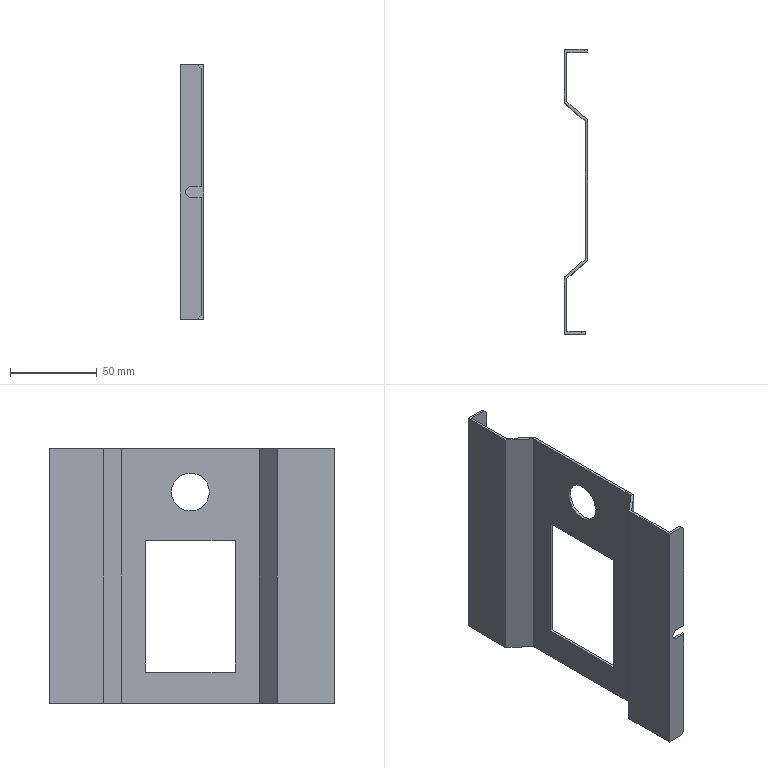Part | SolidWorks | features ICE 4, Chamfer 1, ExtruThin 1, MirrorPattern 1 | 1 solid | 36 faces | box 13.5 x 164.498 x 147 mm | volume 37040 mm3 | plane 29 | cylinder 7 | commonest cylinder face diameters 4.5 x4 22 x2 6 x1
STEP:
#1=CARTESIAN_POINT('',(9.75,162.998,35.));
#2=VERTEX_POINT('',#1);
#3=CARTESIAN_POINT('',(5.25,162.998,35.));
#4=VERTEX_POINT('',#3);
#5=CARTESIAN_POINT('',(7.5,162.998,35.));
#6=DIRECTION('',(0.,1.,0.));
#7=DIRECTION('',(1.,0.,0.));
#8=AXIS2_PLACEMENT_3D('',#5,#6,#7);
#9=CIRCLE('',#8,2.25);
#10=EDGE_CURVE('',#2,#4,#9,.T.);
#11=ORIENTED_EDGE('',*,*,#10,.F.);
#12=CARTESIAN_POINT('',(9.75,164.498,35.));
#13=VERTEX_POINT('',#12);
#14=CARTESIAN_POINT('',(9.75,154.498,35.));
#15=DIRECTION('',(0.,1.,0.));
#16=VECTOR('',#15,1000.);
#17=LINE('',#14,#16);
#18=EDGE_CURVE('',#2,#13,#17,.T.);
#19=ORIENTED_EDGE('',*,*,#18,.T.);
#20=CARTESIAN_POINT('',(5.25,164.498,35.));
#21=VERTEX_POINT('',#20);
#22=CARTESIAN_POINT('',(7.5,164.498,35.));
#23=DIRECTION('',(0.,-1.,0.));
#24=DIRECTION('',(-1.,0.,0.));
#25=AXIS2_PLACEMENT_3D('',#22,#23,#24);
#26=CIRCLE('',#25,2.25);
#27=EDGE_CURVE('',#21,#13,#26,.T.);
#28=ORIENTED_EDGE('',*,*,#27,.F.);
#29=CARTESIAN_POINT('',(5.25,154.498,35.));
#30=DIRECTION('',(0.,1.,0.));
#31=VECTOR('',#30,1000.);
#32=LINE('',#29,#31);
#33=EDGE_CURVE('',#4,#21,#32,.T.);
#34=ORIENTED_EDGE('',*,*,#33,.F.);
#35=EDGE_LOOP('',(#11,#19,#28,#34));
#36=FACE_OUTER_BOUND('',#35,.T.);
#37=CARTESIAN_POINT('',(7.5,154.498,35.));
#38=DIRECTION('',(0.,1.,0.));
#39=DIRECTION('',(-1.,0.,0.));
#40=AXIS2_PLACEMENT_3D('',#37,#38,#39);
#41=CYLINDRICAL_SURFACE('',#40,2.25);
#42=ADVANCED_FACE('',(#36),#41,.F.);
#43=CARTESIAN_POINT('',(5.25,162.998,-35.));
#44=VERTEX_POINT('',#43);
#45=CARTESIAN_POINT('',(9.75,162.998,-35.));
#46=VERTEX_POINT('',#45);
#47=CARTESIAN_POINT('',(7.5,162.998,-35.));
#48=DIRECTION('',(0.,-1.,0.));
#49=DIRECTION('',(1.,0.,0.));
#50=AXIS2_PLACEMENT_3D('',#47,#48,#49);
#51=CIRCLE('',#50,2.25);
#52=EDGE_CURVE('',#44,#46,#51,.T.);
#53=ORIENTED_EDGE('',*,*,#52,.T.);
#54=CARTESIAN_POINT('',(9.75,164.498,-35.));
#55=VERTEX_POINT('',#54);
#56=CARTESIAN_POINT('',(9.75,154.498,-35.));
#57=DIRECTION('',(0.,1.,0.));
#58=VECTOR('',#57,1000.);
#59=LINE('',#56,#58);
#60=EDGE_CURVE('',#46,#55,#59,.T.);
#61=ORIENTED_EDGE('',*,*,#60,.T.);
#62=CARTESIAN_POINT('',(5.25,164.498,-35.));
#63=VERTEX_POINT('',#62);
#64=CARTESIAN_POINT('',(7.5,164.498,-35.));
#65=DIRECTION('',(0.,1.,0.));
#66=DIRECTION('',(-1.,0.,0.));
#67=AXIS2_PLACEMENT_3D('',#64,#65,#66);
#68=CIRCLE('',#67,2.25);
#69=EDGE_CURVE('',#55,#63,#68,.T.);
#70=ORIENTED_EDGE('',*,*,#69,.T.);
#71=CARTESIAN_POINT('',(5.25,154.498,-35.));
#72=DIRECTION('',(0.,1.,0.));
#73=VECTOR('',#72,1000.);
#74=LINE('',#71,#73);
#75=EDGE_CURVE('',#44,#63,#74,.T.);
#76=ORIENTED_EDGE('',*,*,#75,.F.);
#77=EDGE_LOOP('',(#53,#61,#70,#76));
#78=FACE_OUTER_BOUND('',#77,.T.);
#79=CARTESIAN_POINT('',(7.5,154.498,-35.));
#80=DIRECTION('',(0.,1.,0.));
#81=DIRECTION('',(-1.,0.,0.));
#82=AXIS2_PLACEMENT_3D('',#79,#80,#81);
#83=CYLINDRICAL_SURFACE('',#82,2.25);
#84=ADVANCED_FACE('',(#78),#83,.F.);
#85=CARTESIAN_POINT('',(13.5,72.249,48.5));
#86=VERTEX_POINT('',#85);
#87=CARTESIAN_POINT('',(13.5,94.249,48.5));
#88=VERTEX_POINT('',#87);
#89=CARTESIAN_POINT('',(13.5,83.249,48.5));
#90=DIRECTION('',(1.,0.,0.));
#91=DIRECTION('',(0.,1.,0.));
#92=AXIS2_PLACEMENT_3D('',#89,#90,#91);
#93=CIRCLE('',#92,11.);
#94=EDGE_CURVE('',#86,#88,#93,.T.);
#95=ORIENTED_EDGE('',*,*,#94,.T.);
#96=CARTESIAN_POINT('',(12.,94.249,48.5));
#97=VERTEX_POINT('',#96);
#98=CARTESIAN_POINT('',(22.,94.249,48.5));
#99=DIRECTION('',(-1.,0.,0.));
#100=VECTOR('',#99,1000.);
#101=LINE('',#98,#100);
#102=EDGE_CURVE('',#88,#97,#101,.T.);
#103=ORIENTED_EDGE('',*,*,#102,.T.);
#104=CARTESIAN_POINT('',(12.,72.249,48.5));
#105=VERTEX_POINT('',#104);
#106=CARTESIAN_POINT('',(12.,83.249,48.5));
#107=DIRECTION('',(-1.,0.,0.));
#108=DIRECTION('',(0.,-1.,0.));
#109=AXIS2_PLACEMENT_3D('',#106,#107,#108);
#110=CIRCLE('',#109,11.);
#111=EDGE_CURVE('',#97,#105,#110,.T.);
#112=ORIENTED_EDGE('',*,*,#111,.T.);
#113=CARTESIAN_POINT('',(22.,72.249,48.5));
#114=DIRECTION('',(-1.,0.,0.));
#115=VECTOR('',#114,1000.);
#116=LINE('',#113,#115);
#117=EDGE_CURVE('',#86,#105,#116,.T.);
#118=ORIENTED_EDGE('',*,*,#117,.F.);
#119=EDGE_LOOP('',(#95,#103,#112,#118));
#120=FACE_OUTER_BOUND('',#119,.T.);
#121=CARTESIAN_POINT('',(22.,83.249,48.5));
#122=DIRECTION('',(-1.,0.,0.));
#123=DIRECTION('',(0.,-1.,0.));
#124=AXIS2_PLACEMENT_3D('',#121,#122,#123);
#125=CYLINDRICAL_SURFACE('',#124,11.);
#126=ADVANCED_FACE('',(#120),#125,.F.);
#127=CARTESIAN_POINT('',(11.5,162.998,-73.5));
#128=VERTEX_POINT('',#127);
#129=CARTESIAN_POINT('',(1.5,162.998,-73.5));
#130=VERTEX_POINT('',#129);
#131=CARTESIAN_POINT('',(0.,162.998,-73.5));
#132=DIRECTION('',(-1.,0.,0.));
#133=VECTOR('',#132,1000.);
#134=LINE('',#131,#133);
#135=EDGE_CURVE('',#128,#130,#134,.T.);
#136=ORIENTED_EDGE('',*,*,#135,.F.);
#137=CARTESIAN_POINT('',(13.5,162.998,-71.5));
#138=VERTEX_POINT('',#137);
#139=CARTESIAN_POINT('',(79.25,162.998,-5.75));
#140=DIRECTION('',(0.7071,0.,0.7071));
#141=VECTOR('',#140,1000.);
#142=LINE('',#139,#141);
#143=EDGE_CURVE('',#128,#138,#142,.T.);
#144=ORIENTED_EDGE('',*,*,#143,.T.);
#145=CARTESIAN_POINT('',(13.5,162.998,71.5));
#146=VERTEX_POINT('',#145);
#147=CARTESIAN_POINT('',(13.5,162.998,73.5));
#148=DIRECTION('',(0.,0.,-1.));
#149=VECTOR('',#148,1000.);
#150=LINE('',#147,#149);
#151=EDGE_CURVE('',#146,#138,#150,.T.);
#152=ORIENTED_EDGE('',*,*,#151,.F.);
#153=CARTESIAN_POINT('',(11.5,162.998,73.5));
#154=VERTEX_POINT('',#153);
#155=CARTESIAN_POINT('',(5.75,162.998,79.25));
#156=DIRECTION('',(-0.7071,0.,0.7071));
#157=VECTOR('',#156,1000.);
#158=LINE('',#155,#157);
#159=EDGE_CURVE('',#146,#154,#158,.T.);
#160=ORIENTED_EDGE('',*,*,#159,.T.);
#161=CARTESIAN_POINT('',(1.5,162.998,73.5));
#162=VERTEX_POINT('',#161);
#163=CARTESIAN_POINT('',(0.,162.998,73.5));
#164=DIRECTION('',(-1.,0.,0.));
#165=VECTOR('',#164,1000.);
#166=LINE('',#163,#165);
#167=EDGE_CURVE('',#154,#162,#166,.T.);
#168=ORIENTED_EDGE('',*,*,#167,.T.);
#169=CARTESIAN_POINT('',(1.5,162.998,73.5));
#170=DIRECTION('',(0.,0.,-1.));
#171=VECTOR('',#170,1000.);
#172=LINE('',#169,#171);
#173=EDGE_CURVE('',#162,#130,#172,.T.);
#174=ORIENTED_EDGE('',*,*,#173,.T.);
#175=EDGE_LOOP('',(#136,#144,#152,#160,#168,#174));
#176=FACE_OUTER_BOUND('',#175,.T.);
#177=ORIENTED_EDGE('',*,*,#52,.F.);
#178=CARTESIAN_POINT('',(7.5,162.998,-35.));
#179=DIRECTION('',(0.,-1.,0.));
#180=DIRECTION('',(1.,0.,0.));
#181=AXIS2_PLACEMENT_3D('',#178,#179,#180);
#182=CIRCLE('',#181,2.25);
#183=EDGE_CURVE('',#46,#44,#182,.T.);
#184=ORIENTED_EDGE('',*,*,#183,.F.);
#185=EDGE_LOOP('',(#177,#184));
#186=FACE_BOUND('',#185,.T.);
#187=CARTESIAN_POINT('',(7.5,162.998,35.));
#188=DIRECTION('',(0.,1.,0.));
#189=DIRECTION('',(1.,0.,0.));
#190=AXIS2_PLACEMENT_3D('',#187,#188,#189);
#191=CIRCLE('',#190,2.25);
#192=EDGE_CURVE('',#4,#2,#191,.T.);
#193=ORIENTED_EDGE('',*,*,#192,.T.);
#194=ORIENTED_EDGE('',*,*,#10,.T.);
#195=EDGE_LOOP('',(#193,#194));
#196=FACE_BOUND('',#195,.T.);
#197=CARTESIAN_POINT('',(0.,162.998,73.5));
#198=DIRECTION('',(0.,-1.,0.));
#199=DIRECTION('',(1.,0.,0.));
#200=AXIS2_PLACEMENT_3D('',#197,#198,#199);
#201=PLANE('',#200);
#202=ADVANCED_FACE('',(#176,#186,#196),#201,.T.);
#203=CARTESIAN_POINT('',(13.5,164.498,71.5));
#204=VERTEX_POINT('',#203);
#205=CARTESIAN_POINT('',(13.5,164.498,-71.5));
#206=VERTEX_POINT('',#205);
#207=CARTESIAN_POINT('',(13.5,164.498,73.5));
#208=DIRECTION('',(0.,0.,-1.));
#209=VECTOR('',#208,1000.);
#210=LINE('',#207,#209);
#211=EDGE_CURVE('',#204,#206,#210,.T.);
#212=ORIENTED_EDGE('',*,*,#211,.T.);
#213=CARTESIAN_POINT('',(11.5,164.498,-73.5));
#214=VERTEX_POINT('',#213);
#215=CARTESIAN_POINT('',(11.5,164.498,-73.5));
#216=DIRECTION('',(-0.7071,0.,-0.7071));
#217=VECTOR('',#216,1000.);
#218=LINE('',#215,#217);
#219=EDGE_CURVE('',#206,#214,#218,.T.);
#220=ORIENTED_EDGE('',*,*,#219,.T.);
#221=CARTESIAN_POINT('',(0.,164.498,-73.5));
#222=VERTEX_POINT('',#221);
#223=CARTESIAN_POINT('',(0.,164.498,-73.5));
#224=DIRECTION('',(-1.,0.,0.));
#225=VECTOR('',#224,1000.);
#226=LINE('',#223,#225);
#227=EDGE_CURVE('',#214,#222,#226,.T.);
#228=ORIENTED_EDGE('',*,*,#227,.T.);
#229=CARTESIAN_POINT('',(0.,164.498,73.5));
#230=VERTEX_POINT('',#229);
#231=CARTESIAN_POINT('',(0.,164.498,73.5));
#232=DIRECTION('',(0.,0.,-1.));
#233=VECTOR('',#232,1000.);
#234=LINE('',#231,#233);
#235=EDGE_CURVE('',#230,#222,#234,.T.);
#236=ORIENTED_EDGE('',*,*,#235,.F.);
#237=CARTESIAN_POINT('',(11.5,164.498,73.5));
#238=VERTEX_POINT('',#237);
#239=CARTESIAN_POINT('',(0.,164.498,73.5));
#240=DIRECTION('',(-1.,0.,0.));
#241=VECTOR('',#240,1000.);
#242=LINE('',#239,#241);
#243=EDGE_CURVE('',#238,#230,#242,.T.);
#244=ORIENTED_EDGE('',*,*,#243,.F.);
#245=CARTESIAN_POINT('',(13.5,164.498,71.5));
#246=DIRECTION('',(0.7071,0.,-0.7071));
#247=VECTOR('',#246,1000.);
#248=LINE('',#245,#247);
#249=EDGE_CURVE('',#238,#204,#248,.T.);
#250=ORIENTED_EDGE('',*,*,#249,.T.);
#251=EDGE_LOOP('',(#212,#220,#228,#236,#244,#250));
#252=FACE_OUTER_BOUND('',#251,.T.);
#253=CARTESIAN_POINT('',(7.5,164.498,-35.));
#254=DIRECTION('',(0.,1.,0.));
#255=DIRECTION('',(-1.,0.,0.));
#256=AXIS2_PLACEMENT_3D('',#253,#254,#255);
#257=CIRCLE('',#256,2.25);
#258=EDGE_CURVE('',#63,#55,#257,.T.);
#259=ORIENTED_EDGE('',*,*,#258,.F.);
#260=ORIENTED_EDGE('',*,*,#69,.F.);
#261=EDGE_LOOP('',(#259,#260));
#262=FACE_BOUND('',#261,.T.);
#263=ORIENTED_EDGE('',*,*,#27,.T.);
#264=CARTESIAN_POINT('',(7.5,164.498,35.));
#265=DIRECTION('',(0.,-1.,0.));
#266=DIRECTION('',(-1.,0.,0.));
#267=AXIS2_PLACEMENT_3D('',#264,#265,#266);
#268=CIRCLE('',#267,2.25);
#269=EDGE_CURVE('',#13,#21,#268,.T.);
#270=ORIENTED_EDGE('',*,*,#269,.T.);
#271=EDGE_LOOP('',(#263,#270));
#272=FACE_BOUND('',#271,.T.);
#273=CARTESIAN_POINT('',(0.,164.498,73.5));
#274=DIRECTION('',(0.,-1.,0.));
#275=DIRECTION('',(1.,0.,0.));
#276=AXIS2_PLACEMENT_3D('',#273,#274,#275);
#277=PLANE('',#276);
#278=ADVANCED_FACE('',(#252,#262,#272),#277,.F.);
#279=CARTESIAN_POINT('',(12.,1.5,3.));
#280=VERTEX_POINT('',#279);
#281=CARTESIAN_POINT('',(12.,0.,3.));
#282=VERTEX_POINT('',#281);
#283=CARTESIAN_POINT('',(12.,5.,3.));
#284=DIRECTION('',(0.,-1.,0.));
#285=VECTOR('',#284,1000.);
#286=LINE('',#283,#285);
#287=EDGE_CURVE('',#280,#282,#286,.T.);
#288=ORIENTED_EDGE('',*,*,#287,.F.);
#289=CARTESIAN_POINT('',(12.,1.5,71.5));
#290=VERTEX_POINT('',#289);
#291=CARTESIAN_POINT('',(12.,1.5,73.5));
#292=DIRECTION('',(0.,0.,-1.));
#293=VECTOR('',#292,1000.);
#294=LINE('',#291,#293);
#295=EDGE_CURVE('',#290,#280,#294,.T.);
#296=ORIENTED_EDGE('',*,*,#295,.F.);
#297=CARTESIAN_POINT('',(12.,0.,71.5));
#298=VERTEX_POINT('',#297);
#299=CARTESIAN_POINT('',(12.,0.,71.5));
#300=DIRECTION('',(0.,-1.,0.));
#301=VECTOR('',#300,1000.);
#302=LINE('',#299,#301);
#303=EDGE_CURVE('',#290,#298,#302,.T.);
#304=ORIENTED_EDGE('',*,*,#303,.T.);
#305=CARTESIAN_POINT('',(12.,0.,73.5));
#306=DIRECTION('',(0.,0.,-1.));
#307=VECTOR('',#306,1000.);
#308=LINE('',#305,#307);
#309=EDGE_CURVE('',#298,#282,#308,.T.);
#310=ORIENTED_EDGE('',*,*,#309,.T.);
#311=EDGE_LOOP('',(#288,#296,#304,#310));
#312=FACE_OUTER_BOUND('',#311,.T.);
#313=CARTESIAN_POINT('',(12.,1.5,73.5));
#314=DIRECTION('',(1.,0.,0.));
#315=DIRECTION('',(0.,0.,-1.));
#316=AXIS2_PLACEMENT_3D('',#313,#314,#315);
#317=PLANE('',#316);
#318=ADVANCED_FACE('',(#312),#317,.T.);
#319=CARTESIAN_POINT('',(6.,0.,3.));
#320=VERTEX_POINT('',#319);
#321=CARTESIAN_POINT('',(6.,0.,-3.));
#322=VERTEX_POINT('',#321);
#323=CARTESIAN_POINT('',(6.,0.,0.));
#324=DIRECTION('',(0.,-1.,0.));
#325=DIRECTION('',(0.,0.,-1.));
#326=AXIS2_PLACEMENT_3D('',#323,#324,#325);
#327=CIRCLE('',#326,3.);
#328=EDGE_CURVE('',#320,#322,#327,.T.);
#329=ORIENTED_EDGE('',*,*,#328,.F.);
#330=CARTESIAN_POINT('',(6.,0.,3.));
#331=DIRECTION('',(-1.,0.,0.));
#332=VECTOR('',#331,1000.);
#333=LINE('',#330,#332);
#334=EDGE_CURVE('',#282,#320,#333,.T.);
#335=ORIENTED_EDGE('',*,*,#334,.F.);
#336=ORIENTED_EDGE('',*,*,#309,.F.);
#337=CARTESIAN_POINT('',(10.,0.,73.5));
#338=VERTEX_POINT('',#337);
#339=CARTESIAN_POINT('',(12.,0.,71.5));
#340=DIRECTION('',(-0.7071,0.,0.7071));
#341=VECTOR('',#340,1000.);
#342=LINE('',#339,#341);
#343=EDGE_CURVE('',#298,#338,#342,.T.);
#344=ORIENTED_EDGE('',*,*,#343,.T.);
#345=CARTESIAN_POINT('',(0.,0.,73.5));
#346=VERTEX_POINT('',#345);
#347=CARTESIAN_POINT('',(0.,0.,73.5));
#348=DIRECTION('',(1.,0.,0.));
#349=VECTOR('',#348,1000.);
#350=LINE('',#347,#349);
#351=EDGE_CURVE('',#346,#338,#350,.T.);
#352=ORIENTED_EDGE('',*,*,#351,.F.);
#353=CARTESIAN_POINT('',(0.,0.,-73.5));
#354=VERTEX_POINT('',#353);
#355=CARTESIAN_POINT('',(0.,0.,73.5));
#356=DIRECTION('',(0.,0.,-1.));
#357=VECTOR('',#356,1000.);
#358=LINE('',#355,#357);
#359=EDGE_CURVE('',#346,#354,#358,.T.);
#360=ORIENTED_EDGE('',*,*,#359,.T.);
#361=CARTESIAN_POINT('',(10.,0.,-73.5));
#362=VERTEX_POINT('',#361);
#363=CARTESIAN_POINT('',(0.,0.,-73.5));
#364=DIRECTION('',(1.,0.,0.));
#365=VECTOR('',#364,1000.);
#366=LINE('',#363,#365);
#367=EDGE_CURVE('',#354,#362,#366,.T.);
#368=ORIENTED_EDGE('',*,*,#367,.T.);
#369=CARTESIAN_POINT('',(12.,0.,-71.5));
#370=VERTEX_POINT('',#369);
#371=CARTESIAN_POINT('',(10.,0.,-73.5));
#372=DIRECTION('',(0.7071,0.,0.7071));
#373=VECTOR('',#372,1000.);
#374=LINE('',#371,#373);
#375=EDGE_CURVE('',#362,#370,#374,.T.);
#376=ORIENTED_EDGE('',*,*,#375,.T.);
#377=CARTESIAN_POINT('',(12.,0.,-3.));
#378=VERTEX_POINT('',#377);
#379=CARTESIAN_POINT('',(12.,0.,73.5));
#380=DIRECTION('',(0.,0.,-1.));
#381=VECTOR('',#380,1000.);
#382=LINE('',#379,#381);
#383=EDGE_CURVE('',#378,#370,#382,.T.);
#384=ORIENTED_EDGE('',*,*,#383,.F.);
#385=CARTESIAN_POINT('',(6.,0.,-3.));
#386=DIRECTION('',(1.,0.,0.));
#387=VECTOR('',#386,1000.);
#388=LINE('',#385,#387);
#389=EDGE_CURVE('',#322,#378,#388,.T.);
#390=ORIENTED_EDGE('',*,*,#389,.F.);
#391=EDGE_LOOP('',(#329,#335,#336,#344,#352,#360,#368,#376,#384,#390));
#392=FACE_OUTER_BOUND('',#391,.T.);
#393=CARTESIAN_POINT('',(0.,0.,73.5));
#394=DIRECTION('',(0.,1.,0.));
#395=DIRECTION('',(0.,0.,1.));
#396=AXIS2_PLACEMENT_3D('',#393,#394,#395);
#397=PLANE('',#396);
#398=ADVANCED_FACE('',(#392),#397,.F.);
#399=CARTESIAN_POINT('',(12.,1.5,-3.));
#400=VERTEX_POINT('',#399);
#401=CARTESIAN_POINT('',(12.,5.,-3.));
#402=DIRECTION('',(0.,-1.,0.));
#403=VECTOR('',#402,1000.);
#404=LINE('',#401,#403);
#405=EDGE_CURVE('',#400,#378,#404,.T.);
#406=ORIENTED_EDGE('',*,*,#405,.T.);
#407=ORIENTED_EDGE('',*,*,#383,.T.);
#408=CARTESIAN_POINT('',(12.,1.5,-71.5));
#409=VERTEX_POINT('',#408);
#410=CARTESIAN_POINT('',(12.,1.5,-71.5));
#411=DIRECTION('',(0.,1.,0.));
#412=VECTOR('',#411,1000.);
#413=LINE('',#410,#412);
#414=EDGE_CURVE('',#370,#409,#413,.T.);
#415=ORIENTED_EDGE('',*,*,#414,.T.);
#416=CARTESIAN_POINT('',(12.,1.5,73.5));
#417=DIRECTION('',(0.,0.,-1.));
#418=VECTOR('',#417,1000.);
#419=LINE('',#416,#418);
#420=EDGE_CURVE('',#400,#409,#419,.T.);
#421=ORIENTED_EDGE('',*,*,#420,.F.);
#422=EDGE_LOOP('',(#406,#407,#415,#421));
#423=FACE_OUTER_BOUND('',#422,.T.);
#424=CARTESIAN_POINT('',(12.,1.5,73.5));
#425=DIRECTION('',(1.,0.,0.));
#426=DIRECTION('',(0.,0.,-1.));
#427=AXIS2_PLACEMENT_3D('',#424,#425,#426);
#428=PLANE('',#427);
#429=ADVANCED_FACE('',(#423),#428,.T.);
#430=CARTESIAN_POINT('',(6.,1.5,3.));
#431=VERTEX_POINT('',#430);
#432=CARTESIAN_POINT('',(0.,1.5,3.));
#433=DIRECTION('',(1.,0.,0.));
#434=VECTOR('',#433,1000.);
#435=LINE('',#432,#434);
#436=EDGE_CURVE('',#431,#280,#435,.T.);
#437=ORIENTED_EDGE('',*,*,#436,.F.);
#438=CARTESIAN_POINT('',(6.,1.5,-3.));
#439=VERTEX_POINT('',#438);
#440=CARTESIAN_POINT('',(6.,1.5,0.));
#441=DIRECTION('',(0.,1.,0.));
#442=DIRECTION('',(0.,0.,1.));
#443=AXIS2_PLACEMENT_3D('',#440,#441,#442);
#444=CIRCLE('',#443,3.);
#445=EDGE_CURVE('',#439,#431,#444,.T.);
#446=ORIENTED_EDGE('',*,*,#445,.F.);
#447=CARTESIAN_POINT('',(0.,1.5,-3.));
#448=DIRECTION('',(-1.,0.,0.));
#449=VECTOR('',#448,1000.);
#450=LINE('',#447,#449);
#451=EDGE_CURVE('',#400,#439,#450,.T.);
#452=ORIENTED_EDGE('',*,*,#451,.F.);
#453=ORIENTED_EDGE('',*,*,#420,.T.);
#454=CARTESIAN_POINT('',(10.,1.5,-73.5));
#455=VERTEX_POINT('',#454);
#456=CARTESIAN_POINT('',(78.5,1.5,-5.));
#457=DIRECTION('',(-0.7071,0.,-0.7071));
#458=VECTOR('',#457,1000.);
#459=LINE('',#456,#458);
#460=EDGE_CURVE('',#409,#455,#459,.T.);
#461=ORIENTED_EDGE('',*,*,#460,.T.);
#462=CARTESIAN_POINT('',(1.5,1.5,-73.5));
#463=VERTEX_POINT('',#462);
#464=CARTESIAN_POINT('',(0.,1.5,-73.5));
#465=DIRECTION('',(1.,0.,0.));
#466=VECTOR('',#465,1000.);
#467=LINE('',#464,#466);
#468=EDGE_CURVE('',#463,#455,#467,.T.);
#469=ORIENTED_EDGE('',*,*,#468,.F.);
#470=CARTESIAN_POINT('',(1.5,1.5,73.5));
#471=VERTEX_POINT('',#470);
#472=CARTESIAN_POINT('',(1.5,1.5,73.5));
#473=DIRECTION('',(0.,0.,-1.));
#474=VECTOR('',#473,1000.);
#475=LINE('',#472,#474);
#476=EDGE_CURVE('',#471,#463,#475,.T.);
#477=ORIENTED_EDGE('',*,*,#476,.F.);
#478=CARTESIAN_POINT('',(10.,1.5,73.5));
#479=VERTEX_POINT('',#478);
#480=CARTESIAN_POINT('',(0.,1.5,73.5));
#481=DIRECTION('',(1.,0.,0.));
#482=VECTOR('',#481,1000.);
#483=LINE('',#480,#482);
#484=EDGE_CURVE('',#471,#479,#483,.T.);
#485=ORIENTED_EDGE('',*,*,#484,.T.);
#486=CARTESIAN_POINT('',(5.,1.5,78.5));
#487=DIRECTION('',(0.7071,0.,-0.7071));
#488=VECTOR('',#487,1000.);
#489=LINE('',#486,#488);
#490=EDGE_CURVE('',#479,#290,#489,.T.);
#491=ORIENTED_EDGE('',*,*,#490,.T.);
#492=ORIENTED_EDGE('',*,*,#295,.T.);
#493=EDGE_LOOP('',(#437,#446,#452,#453,#461,#469,#477,#485,#491,#492));
#494=FACE_OUTER_BOUND('',#493,.T.);
#495=CARTESIAN_POINT('',(0.,1.5,73.5));
#496=DIRECTION('',(0.,1.,0.));
#497=DIRECTION('',(0.,0.,1.));
#498=AXIS2_PLACEMENT_3D('',#495,#496,#497);
#499=PLANE('',#498);
#500=ADVANCED_FACE('',(#494),#499,.T.);
#501=CARTESIAN_POINT('',(1.5,32.308,-73.5));
#502=VERTEX_POINT('',#501);
#503=CARTESIAN_POINT('',(1.5,0.,-73.5));
#504=DIRECTION('',(0.,-1.,0.));
#505=VECTOR('',#504,1000.);
#506=LINE('',#503,#505);
#507=EDGE_CURVE('',#502,#463,#506,.T.);
#508=ORIENTED_EDGE('',*,*,#507,.F.);
#509=CARTESIAN_POINT('',(1.5,32.308,73.5));
#510=VERTEX_POINT('',#509);
#511=CARTESIAN_POINT('',(1.5,32.308,73.5));
#512=DIRECTION('',(0.,0.,-1.));
#513=VECTOR('',#512,1000.);
#514=LINE('',#511,#513);
#515=EDGE_CURVE('',#510,#502,#514,.T.);
#516=ORIENTED_EDGE('',*,*,#515,.F.);
#517=CARTESIAN_POINT('',(1.5,0.,73.5));
#518=DIRECTION('',(0.,-1.,0.));
#519=VECTOR('',#518,1000.);
#520=LINE('',#517,#519);
#521=EDGE_CURVE('',#510,#471,#520,.T.);
#522=ORIENTED_EDGE('',*,*,#521,.T.);
#523=ORIENTED_EDGE('',*,*,#476,.T.);
#524=EDGE_LOOP('',(#508,#516,#522,#523));
#525=FACE_OUTER_BOUND('',#524,.T.);
#526=CARTESIAN_POINT('',(1.5,0.,73.5));
#527=DIRECTION('',(1.,0.,0.));
#528=DIRECTION('',(0.,0.,-1.));
#529=AXIS2_PLACEMENT_3D('',#526,#527,#528);
#530=PLANE('',#529);
#531=ADVANCED_FACE('',(#525),#530,.T.);
#532=CARTESIAN_POINT('',(13.5,42.557,-73.5));
#533=VERTEX_POINT('',#532);
#534=CARTESIAN_POINT('',(0.9742,31.859,-73.5));
#535=DIRECTION('',(-0.7604,-0.6494,0.));
#536=VECTOR('',#535,1000.);
#537=LINE('',#534,#536);
#538=EDGE_CURVE('',#533,#502,#537,.T.);
#539=ORIENTED_EDGE('',*,*,#538,.F.);
#540=CARTESIAN_POINT('',(13.5,42.557,73.5));
#541=VERTEX_POINT('',#540);
#542=CARTESIAN_POINT('',(13.5,42.557,73.5));
#543=DIRECTION('',(0.,0.,-1.));
#544=VECTOR('',#543,1000.);
#545=LINE('',#542,#544);
#546=EDGE_CURVE('',#541,#533,#545,.T.);
#547=ORIENTED_EDGE('',*,*,#546,.F.);
#548=CARTESIAN_POINT('',(0.9742,31.859,73.5));
#549=DIRECTION('',(-0.7604,-0.6494,0.));
#550=VECTOR('',#549,1000.);
#551=LINE('',#548,#550);
#552=EDGE_CURVE('',#541,#510,#551,.T.);
#553=ORIENTED_EDGE('',*,*,#552,.T.);
#554=ORIENTED_EDGE('',*,*,#515,.T.);
#555=EDGE_LOOP('',(#539,#547,#553,#554));
#556=FACE_OUTER_BOUND('',#555,.T.);
#557=CARTESIAN_POINT('',(0.9742,31.859,73.5));
#558=DIRECTION('',(0.6494,-0.7604,0.));
#559=DIRECTION('',(0.7604,0.6494,0.));
#560=AXIS2_PLACEMENT_3D('',#557,#558,#559);
#561=PLANE('',#560);
#562=ADVANCED_FACE('',(#556),#561,.T.);
#563=ORIENTED_EDGE('',*,*,#94,.F.);
#564=CARTESIAN_POINT('',(13.5,83.249,48.5));
#565=DIRECTION('',(1.,0.,0.));
#566=DIRECTION('',(0.,1.,0.));
#567=AXIS2_PLACEMENT_3D('',#564,#565,#566);
#568=CIRCLE('',#567,11.);
#569=EDGE_CURVE('',#88,#86,#568,.T.);
#570=ORIENTED_EDGE('',*,*,#569,.F.);
#571=EDGE_LOOP('',(#563,#570));
#572=FACE_BOUND('',#571,.T.);
#573=CARTESIAN_POINT('',(13.5,57.249,-55.5));
#574=VERTEX_POINT('',#573);
#575=CARTESIAN_POINT('',(13.5,109.249,-55.5));
#576=VERTEX_POINT('',#575);
#577=CARTESIAN_POINT('',(13.5,43.249,-55.5));
#578=DIRECTION('',(0.,1.,0.));
#579=VECTOR('',#578,1000.);
#580=LINE('',#577,#579);
#581=EDGE_CURVE('',#574,#576,#580,.T.);
#582=ORIENTED_EDGE('',*,*,#581,.F.);
#583=CARTESIAN_POINT('',(13.5,57.249,20.5));
#584=VERTEX_POINT('',#583);
#585=CARTESIAN_POINT('',(13.5,57.249,73.5));
#586=DIRECTION('',(0.,0.,-1.));
#587=VECTOR('',#586,1000.);
#588=LINE('',#585,#587);
#589=EDGE_CURVE('',#584,#574,#588,.T.);
#590=ORIENTED_EDGE('',*,*,#589,.F.);
#591=CARTESIAN_POINT('',(13.5,109.249,20.5));
#592=VERTEX_POINT('',#591);
#593=CARTESIAN_POINT('',(13.5,43.249,20.5));
#594=DIRECTION('',(0.,-1.,0.));
#595=VECTOR('',#594,1000.);
#596=LINE('',#593,#595);
#597=EDGE_CURVE('',#592,#584,#596,.T.);
#598=ORIENTED_EDGE('',*,*,#597,.F.);
#599=CARTESIAN_POINT('',(13.5,109.249,73.5));
#600=DIRECTION('',(0.,0.,1.));
#601=VECTOR('',#600,1000.);
#602=LINE('',#599,#601);
#603=EDGE_CURVE('',#576,#592,#602,.T.);
#604=ORIENTED_EDGE('',*,*,#603,.F.);
#605=EDGE_LOOP('',(#582,#590,#598,#604));
#606=FACE_BOUND('',#605,.T.);
#607=CARTESIAN_POINT('',(13.5,123.94,-73.5));
#608=VERTEX_POINT('',#607);
#609=CARTESIAN_POINT('',(13.5,43.249,-73.5));
#610=DIRECTION('',(0.,-1.,0.));
#611=VECTOR('',#610,1000.);
#612=LINE('',#609,#611);
#613=EDGE_CURVE('',#608,#533,#612,.T.);
#614=ORIENTED_EDGE('',*,*,#613,.F.);
#615=CARTESIAN_POINT('',(13.5,123.94,73.5));
#616=VERTEX_POINT('',#615);
#617=CARTESIAN_POINT('',(13.5,123.94,73.5));
#618=DIRECTION('',(0.,0.,-1.));
#619=VECTOR('',#618,1000.);
#620=LINE('',#617,#619);
#621=EDGE_CURVE('',#616,#608,#620,.T.);
#622=ORIENTED_EDGE('',*,*,#621,.F.);
#623=CARTESIAN_POINT('',(13.5,43.249,73.5));
#624=DIRECTION('',(0.,-1.,0.));
#625=VECTOR('',#624,1000.);
#626=LINE('',#623,#625);
#627=EDGE_CURVE('',#616,#541,#626,.T.);
#628=ORIENTED_EDGE('',*,*,#627,.T.);
#629=ORIENTED_EDGE('',*,*,#546,.T.);
#630=EDGE_LOOP('',(#614,#622,#628,#629));
#631=FACE_OUTER_BOUND('',#630,.T.);
#632=CARTESIAN_POINT('',(13.5,43.249,73.5));
#633=DIRECTION('',(1.,0.,0.));
#634=DIRECTION('',(0.,1.,0.));
#635=AXIS2_PLACEMENT_3D('',#632,#633,#634);
#636=PLANE('',#635);
#637=ADVANCED_FACE('',(#572,#606,#631),#636,.T.);
#638=CARTESIAN_POINT('',(1.5,134.189,-73.5));
#639=VERTEX_POINT('',#638);
#640=CARTESIAN_POINT('',(12.974,124.39,-73.5));
#641=DIRECTION('',(0.7604,-0.6494,0.));
#642=VECTOR('',#641,1000.);
#643=LINE('',#640,#642);
#644=EDGE_CURVE('',#639,#608,#643,.T.);
#645=ORIENTED_EDGE('',*,*,#644,.F.);
#646=CARTESIAN_POINT('',(1.5,134.189,73.5));
#647=VERTEX_POINT('',#646);
#648=CARTESIAN_POINT('',(1.5,134.189,73.5));
#649=DIRECTION('',(0.,0.,-1.));
#650=VECTOR('',#649,1000.);
#651=LINE('',#648,#650);
#652=EDGE_CURVE('',#647,#639,#651,.T.);
#653=ORIENTED_EDGE('',*,*,#652,.F.);
#654=CARTESIAN_POINT('',(12.974,124.39,73.5));
#655=DIRECTION('',(0.7604,-0.6494,0.));
#656=VECTOR('',#655,1000.);
#657=LINE('',#654,#656);
#658=EDGE_CURVE('',#647,#616,#657,.T.);
#659=ORIENTED_EDGE('',*,*,#658,.T.);
#660=ORIENTED_EDGE('',*,*,#621,.T.);
#661=EDGE_LOOP('',(#645,#653,#659,#660));
#662=FACE_OUTER_BOUND('',#661,.T.);
#663=CARTESIAN_POINT('',(12.974,124.39,73.5));
#664=DIRECTION('',(0.6494,0.7604,0.));
#665=DIRECTION('',(-0.7604,0.6494,0.));
#666=AXIS2_PLACEMENT_3D('',#663,#664,#665);
#667=PLANE('',#666);
#668=ADVANCED_FACE('',(#662),#667,.T.);
#669=CARTESIAN_POINT('',(1.5,133.498,-73.5));
#670=DIRECTION('',(0.,-1.,0.));
#671=VECTOR('',#670,1000.);
#672=LINE('',#669,#671);
#673=EDGE_CURVE('',#130,#639,#672,.T.);
#674=ORIENTED_EDGE('',*,*,#673,.F.);
#675=ORIENTED_EDGE('',*,*,#173,.F.);
#676=CARTESIAN_POINT('',(1.5,133.498,73.5));
#677=DIRECTION('',(0.,-1.,0.));
#678=VECTOR('',#677,1000.);
#679=LINE('',#676,#678);
#680=EDGE_CURVE('',#162,#647,#679,.T.);
#681=ORIENTED_EDGE('',*,*,#680,.T.);
#682=ORIENTED_EDGE('',*,*,#652,.T.);
#683=EDGE_LOOP('',(#674,#675,#681,#682));
#684=FACE_OUTER_BOUND('',#683,.T.);
#685=CARTESIAN_POINT('',(1.5,133.498,73.5));
#686=DIRECTION('',(1.,0.,0.));
#687=DIRECTION('',(0.,1.,0.));
#688=AXIS2_PLACEMENT_3D('',#685,#686,#687);
#689=PLANE('',#688);
#690=ADVANCED_FACE('',(#684),#689,.T.);
#691=ORIENTED_EDGE('',*,*,#151,.T.);
#692=CARTESIAN_POINT('',(13.5,164.498,-71.5));
#693=DIRECTION('',(0.,1.,0.));
#694=VECTOR('',#693,1000.);
#695=LINE('',#692,#694);
#696=EDGE_CURVE('',#138,#206,#695,.T.);
#697=ORIENTED_EDGE('',*,*,#696,.T.);
#698=ORIENTED_EDGE('',*,*,#211,.F.);
#699=CARTESIAN_POINT('',(13.5,162.998,71.5));
#700=DIRECTION('',(0.,-1.,0.));
#701=VECTOR('',#700,1000.);
#702=LINE('',#699,#701);
#703=EDGE_CURVE('',#204,#146,#702,.T.);
#704=ORIENTED_EDGE('',*,*,#703,.T.);
#705=EDGE_LOOP('',(#691,#697,#698,#704));
#706=FACE_OUTER_BOUND('',#705,.T.);
#707=CARTESIAN_POINT('',(13.5,164.498,73.5));
#708=DIRECTION('',(1.,0.,0.));
#709=DIRECTION('',(0.,1.,0.));
#710=AXIS2_PLACEMENT_3D('',#707,#708,#709);
#711=PLANE('',#710);
#712=ADVANCED_FACE('',(#706),#711,.T.);
#713=CARTESIAN_POINT('',(0.,133.498,-73.5));
#714=VERTEX_POINT('',#713);
#715=CARTESIAN_POINT('',(0.,133.498,-73.5));
#716=DIRECTION('',(0.,-1.,0.));
#717=VECTOR('',#716,1000.);
#718=LINE('',#715,#717);
#719=EDGE_CURVE('',#222,#714,#718,.T.);
#720=ORIENTED_EDGE('',*,*,#719,.T.);
#721=CARTESIAN_POINT('',(0.,133.498,73.5));
#722=VERTEX_POINT('',#721);
#723=CARTESIAN_POINT('',(0.,133.498,73.5));
#724=DIRECTION('',(0.,0.,-1.));
#725=VECTOR('',#724,1000.);
#726=LINE('',#723,#725);
#727=EDGE_CURVE('',#722,#714,#726,.T.);
#728=ORIENTED_EDGE('',*,*,#727,.F.);
#729=CARTESIAN_POINT('',(0.,133.498,73.5));
#730=DIRECTION('',(0.,-1.,0.));
#731=VECTOR('',#730,1000.);
#732=LINE('',#729,#731);
#733=EDGE_CURVE('',#230,#722,#732,.T.);
#734=ORIENTED_EDGE('',*,*,#733,.F.);
#735=ORIENTED_EDGE('',*,*,#235,.T.);
#736=EDGE_LOOP('',(#720,#728,#734,#735));
#737=FACE_OUTER_BOUND('',#736,.T.);
#738=CARTESIAN_POINT('',(0.,133.498,73.5));
#739=DIRECTION('',(1.,0.,0.));
#740=DIRECTION('',(0.,1.,0.));
#741=AXIS2_PLACEMENT_3D('',#738,#739,#740);
#742=PLANE('',#741);
#743=ADVANCED_FACE('',(#737),#742,.F.);
#744=CARTESIAN_POINT('',(12.,123.249,-73.5));
#745=VERTEX_POINT('',#744);
#746=CARTESIAN_POINT('',(12.,123.249,-73.5));
#747=DIRECTION('',(0.7604,-0.6494,0.));
#748=VECTOR('',#747,1000.);
#749=LINE('',#746,#748);
#750=EDGE_CURVE('',#714,#745,#749,.T.);
#751=ORIENTED_EDGE('',*,*,#750,.T.);
#752=CARTESIAN_POINT('',(12.,123.249,73.5));
#753=VERTEX_POINT('',#752);
#754=CARTESIAN_POINT('',(12.,123.249,73.5));
#755=DIRECTION('',(0.,0.,-1.));
#756=VECTOR('',#755,1000.);
#757=LINE('',#754,#756);
#758=EDGE_CURVE('',#753,#745,#757,.T.);
#759=ORIENTED_EDGE('',*,*,#758,.F.);
#760=CARTESIAN_POINT('',(12.,123.249,73.5));
#761=DIRECTION('',(0.7604,-0.6494,0.));
#762=VECTOR('',#761,1000.);
#763=LINE('',#760,#762);
#764=EDGE_CURVE('',#722,#753,#763,.T.);
#765=ORIENTED_EDGE('',*,*,#764,.F.);
#766=ORIENTED_EDGE('',*,*,#727,.T.);
#767=EDGE_LOOP('',(#751,#759,#765,#766));
#768=FACE_OUTER_BOUND('',#767,.T.);
#769=CARTESIAN_POINT('',(12.,123.249,73.5));
#770=DIRECTION('',(0.6494,0.7604,0.));
#771=DIRECTION('',(-0.7604,0.6494,0.));
#772=AXIS2_PLACEMENT_3D('',#769,#770,#771);
#773=PLANE('',#772);
#774=ADVANCED_FACE('',(#768),#773,.F.);
#775=CARTESIAN_POINT('',(12.,83.249,48.5));
#776=DIRECTION('',(-1.,0.,0.));
#777=DIRECTION('',(0.,-1.,0.));
#778=AXIS2_PLACEMENT_3D('',#775,#776,#777);
#779=CIRCLE('',#778,11.);
#780=EDGE_CURVE('',#105,#97,#779,.T.);
#781=ORIENTED_EDGE('',*,*,#780,.F.);
#782=ORIENTED_EDGE('',*,*,#111,.F.);
#783=EDGE_LOOP('',(#781,#782));
#784=FACE_BOUND('',#783,.T.);
#785=CARTESIAN_POINT('',(12.,57.249,-55.5));
#786=VERTEX_POINT('',#785);
#787=CARTESIAN_POINT('',(12.,57.249,20.5));
#788=VERTEX_POINT('',#787);
#789=CARTESIAN_POINT('',(12.,57.249,-55.5));
#790=DIRECTION('',(0.,0.,1.));
#791=VECTOR('',#790,1000.);
#792=LINE('',#789,#791);
#793=EDGE_CURVE('',#786,#788,#792,.T.);
#794=ORIENTED_EDGE('',*,*,#793,.F.);
#795=CARTESIAN_POINT('',(12.,109.249,-55.5));
#796=VERTEX_POINT('',#795);
#797=CARTESIAN_POINT('',(12.,109.249,-55.5));
#798=DIRECTION('',(0.,-1.,0.));
#799=VECTOR('',#798,1000.);
#800=LINE('',#797,#799);
#801=EDGE_CURVE('',#796,#786,#800,.T.);
#802=ORIENTED_EDGE('',*,*,#801,.F.);
#803=CARTESIAN_POINT('',(12.,109.249,20.5));
#804=VERTEX_POINT('',#803);
#805=CARTESIAN_POINT('',(12.,109.249,-55.5));
#806=DIRECTION('',(0.,0.,-1.));
#807=VECTOR('',#806,1000.);
#808=LINE('',#805,#807);
#809=EDGE_CURVE('',#804,#796,#808,.T.);
#810=ORIENTED_EDGE('',*,*,#809,.F.);
#811=CARTESIAN_POINT('',(12.,109.249,20.5));
#812=DIRECTION('',(0.,1.,0.));
#813=VECTOR('',#812,1000.);
#814=LINE('',#811,#813);
#815=EDGE_CURVE('',#788,#804,#814,.T.);
#816=ORIENTED_EDGE('',*,*,#815,.F.);
#817=EDGE_LOOP('',(#794,#802,#810,#816));
#818=FACE_BOUND('',#817,.T.);
#819=CARTESIAN_POINT('',(12.,43.249,-73.5));
#820=VERTEX_POINT('',#819);
#821=CARTESIAN_POINT('',(12.,43.249,-73.5));
#822=DIRECTION('',(0.,-1.,0.));
#823=VECTOR('',#822,1000.);
#824=LINE('',#821,#823);
#825=EDGE_CURVE('',#745,#820,#824,.T.);
#826=ORIENTED_EDGE('',*,*,#825,.T.);
#827=CARTESIAN_POINT('',(12.,43.249,73.5));
#828=VERTEX_POINT('',#827);
#829=CARTESIAN_POINT('',(12.,43.249,73.5));
#830=DIRECTION('',(0.,0.,-1.));
#831=VECTOR('',#830,1000.);
#832=LINE('',#829,#831);
#833=EDGE_CURVE('',#828,#820,#832,.T.);
#834=ORIENTED_EDGE('',*,*,#833,.F.);
#835=CARTESIAN_POINT('',(12.,43.249,73.5));
#836=DIRECTION('',(0.,-1.,0.));
#837=VECTOR('',#836,1000.);
#838=LINE('',#835,#837);
#839=EDGE_CURVE('',#753,#828,#838,.T.);
#840=ORIENTED_EDGE('',*,*,#839,.F.);
#841=ORIENTED_EDGE('',*,*,#758,.T.);
#842=EDGE_LOOP('',(#826,#834,#840,#841));
#843=FACE_OUTER_BOUND('',#842,.T.);
#844=CARTESIAN_POINT('',(12.,43.249,73.5));
#845=DIRECTION('',(1.,0.,0.));
#846=DIRECTION('',(0.,1.,0.));
#847=AXIS2_PLACEMENT_3D('',#844,#845,#846);
#848=PLANE('',#847);
#849=ADVANCED_FACE('',(#784,#818,#843),#848,.F.);
#850=CARTESIAN_POINT('',(0.,33.,-73.5));
#851=VERTEX_POINT('',#850);
#852=CARTESIAN_POINT('',(0.,33.,-73.5));
#853=DIRECTION('',(-0.7604,-0.6494,0.));
#854=VECTOR('',#853,1000.);
#855=LINE('',#852,#854);
#856=EDGE_CURVE('',#820,#851,#855,.T.);
#857=ORIENTED_EDGE('',*,*,#856,.T.);
#858=CARTESIAN_POINT('',(0.,33.,73.5));
#859=VERTEX_POINT('',#858);
#860=CARTESIAN_POINT('',(0.,33.,73.5));
#861=DIRECTION('',(0.,0.,-1.));
#862=VECTOR('',#861,1000.);
#863=LINE('',#860,#862);
#864=EDGE_CURVE('',#859,#851,#863,.T.);
#865=ORIENTED_EDGE('',*,*,#864,.F.);
#866=CARTESIAN_POINT('',(0.,33.,73.5));
#867=DIRECTION('',(-0.7604,-0.6494,0.));
#868=VECTOR('',#867,1000.);
#869=LINE('',#866,#868);
#870=EDGE_CURVE('',#828,#859,#869,.T.);
#871=ORIENTED_EDGE('',*,*,#870,.F.);
#872=ORIENTED_EDGE('',*,*,#833,.T.);
#873=EDGE_LOOP('',(#857,#865,#871,#872));
#874=FACE_OUTER_BOUND('',#873,.T.);
#875=CARTESIAN_POINT('',(0.,33.,73.5));
#876=DIRECTION('',(0.6494,-0.7604,0.));
#877=DIRECTION('',(0.7604,0.6494,0.));
#878=AXIS2_PLACEMENT_3D('',#875,#876,#877);
#879=PLANE('',#878);
#880=ADVANCED_FACE('',(#874),#879,.F.);
#881=CARTESIAN_POINT('',(0.,0.,-73.5));
#882=DIRECTION('',(0.,-1.,0.));
#883=VECTOR('',#882,1000.);
#884=LINE('',#881,#883);
#885=EDGE_CURVE('',#851,#354,#884,.T.);
#886=ORIENTED_EDGE('',*,*,#885,.T.);
#887=ORIENTED_EDGE('',*,*,#359,.F.);
#888=CARTESIAN_POINT('',(0.,0.,73.5));
#889=DIRECTION('',(0.,-1.,0.));
#890=VECTOR('',#889,1000.);
#891=LINE('',#888,#890);
#892=EDGE_CURVE('',#859,#346,#891,.T.);
#893=ORIENTED_EDGE('',*,*,#892,.F.);
#894=ORIENTED_EDGE('',*,*,#864,.T.);
#895=EDGE_LOOP('',(#886,#887,#893,#894));
#896=FACE_OUTER_BOUND('',#895,.T.);
#897=CARTESIAN_POINT('',(0.,0.,73.5));
#898=DIRECTION('',(1.,0.,0.));
#899=DIRECTION('',(0.,0.,-1.));
#900=AXIS2_PLACEMENT_3D('',#897,#898,#899);
#901=PLANE('',#900);
#902=ADVANCED_FACE('',(#896),#901,.F.);
#903=ORIENTED_EDGE('',*,*,#351,.T.);
#904=CARTESIAN_POINT('',(10.,1.5,73.5));
#905=DIRECTION('',(0.,1.,0.));
#906=VECTOR('',#905,1000.);
#907=LINE('',#904,#906);
#908=EDGE_CURVE('',#338,#479,#907,.T.);
#909=ORIENTED_EDGE('',*,*,#908,.T.);
#910=ORIENTED_EDGE('',*,*,#484,.F.);
#911=ORIENTED_EDGE('',*,*,#521,.F.);
#912=ORIENTED_EDGE('',*,*,#552,.F.);
#913=ORIENTED_EDGE('',*,*,#627,.F.);
#914=ORIENTED_EDGE('',*,*,#658,.F.);
#915=ORIENTED_EDGE('',*,*,#680,.F.);
#916=ORIENTED_EDGE('',*,*,#167,.F.);
#917=CARTESIAN_POINT('',(11.5,164.498,73.5));
#918=DIRECTION('',(0.,1.,0.));
#919=VECTOR('',#918,1000.);
#920=LINE('',#917,#919);
#921=EDGE_CURVE('',#154,#238,#920,.T.);
#922=ORIENTED_EDGE('',*,*,#921,.T.);
#923=ORIENTED_EDGE('',*,*,#243,.T.);
#924=ORIENTED_EDGE('',*,*,#733,.T.);
#925=ORIENTED_EDGE('',*,*,#764,.T.);
#926=ORIENTED_EDGE('',*,*,#839,.T.);
#927=ORIENTED_EDGE('',*,*,#870,.T.);
#928=ORIENTED_EDGE('',*,*,#892,.T.);
#929=EDGE_LOOP('',(#903,#909,#910,#911,#912,#913,#914,#915,#916,#922,#923,#924,#925,#926,#927,#928));
#930=FACE_OUTER_BOUND('',#929,.T.);
#931=CARTESIAN_POINT('',(12.,0.,73.5));
#932=DIRECTION('',(0.,0.,-1.));
#933=DIRECTION('',(-1.,0.,0.));
#934=AXIS2_PLACEMENT_3D('',#931,#932,#933);
#935=PLANE('',#934);
#936=ADVANCED_FACE('',(#930),#935,.F.);
#937=ORIENTED_EDGE('',*,*,#468,.T.);
#938=CARTESIAN_POINT('',(10.,0.,-73.5));
#939=DIRECTION('',(0.,-1.,0.));
#940=VECTOR('',#939,1000.);
#941=LINE('',#938,#940);
#942=EDGE_CURVE('',#455,#362,#941,.T.);
#943=ORIENTED_EDGE('',*,*,#942,.T.);
#944=ORIENTED_EDGE('',*,*,#367,.F.);
#945=ORIENTED_EDGE('',*,*,#885,.F.);
#946=ORIENTED_EDGE('',*,*,#856,.F.);
#947=ORIENTED_EDGE('',*,*,#825,.F.);
#948=ORIENTED_EDGE('',*,*,#750,.F.);
#949=ORIENTED_EDGE('',*,*,#719,.F.);
#950=ORIENTED_EDGE('',*,*,#227,.F.);
#951=CARTESIAN_POINT('',(11.5,0.,-73.5));
#952=DIRECTION('',(0.,-1.,0.));
#953=VECTOR('',#952,1000.);
#954=LINE('',#951,#953);
#955=EDGE_CURVE('',#214,#128,#954,.T.);
#956=ORIENTED_EDGE('',*,*,#955,.T.);
#957=ORIENTED_EDGE('',*,*,#135,.T.);
#958=ORIENTED_EDGE('',*,*,#673,.T.);
#959=ORIENTED_EDGE('',*,*,#644,.T.);
#960=ORIENTED_EDGE('',*,*,#613,.T.);
#961=ORIENTED_EDGE('',*,*,#538,.T.);
#962=ORIENTED_EDGE('',*,*,#507,.T.);
#963=EDGE_LOOP('',(#937,#943,#944,#945,#946,#947,#948,#949,#950,#956,#957,#958,#959,#960,#961,#962));
#964=FACE_OUTER_BOUND('',#963,.T.);
#965=CARTESIAN_POINT('',(12.,0.,-73.5));
#966=DIRECTION('',(0.,0.,-1.));
#967=DIRECTION('',(-1.,0.,0.));
#968=AXIS2_PLACEMENT_3D('',#965,#966,#967);
#969=PLANE('',#968);
#970=ADVANCED_FACE('',(#964),#969,.T.);
#971=ORIENTED_EDGE('',*,*,#581,.T.);
#972=CARTESIAN_POINT('',(22.,109.249,-55.5));
#973=DIRECTION('',(-1.,0.,0.));
#974=VECTOR('',#973,1000.);
#975=LINE('',#972,#974);
#976=EDGE_CURVE('',#576,#796,#975,.T.);
#977=ORIENTED_EDGE('',*,*,#976,.T.);
#978=ORIENTED_EDGE('',*,*,#801,.T.);
#979=CARTESIAN_POINT('',(22.,57.249,-55.5));
#980=DIRECTION('',(-1.,0.,0.));
#981=VECTOR('',#980,1000.);
#982=LINE('',#979,#981);
#983=EDGE_CURVE('',#574,#786,#982,.T.);
#984=ORIENTED_EDGE('',*,*,#983,.F.);
#985=EDGE_LOOP('',(#971,#977,#978,#984));
#986=FACE_OUTER_BOUND('',#985,.T.);
#987=CARTESIAN_POINT('',(22.,109.249,-55.5));
#988=DIRECTION('',(0.,0.,-1.));
#989=DIRECTION('',(0.,1.,0.));
#990=AXIS2_PLACEMENT_3D('',#987,#988,#989);
#991=PLANE('',#990);
#992=ADVANCED_FACE('',(#986),#991,.F.);
#993=ORIENTED_EDGE('',*,*,#603,.T.);
#994=CARTESIAN_POINT('',(22.,109.249,20.5));
#995=DIRECTION('',(-1.,0.,0.));
#996=VECTOR('',#995,1000.);
#997=LINE('',#994,#996);
#998=EDGE_CURVE('',#592,#804,#997,.T.);
#999=ORIENTED_EDGE('',*,*,#998,.T.);
#1000=ORIENTED_EDGE('',*,*,#809,.T.);
#1001=ORIENTED_EDGE('',*,*,#976,.F.);
#1002=EDGE_LOOP('',(#993,#999,#1000,#1001));
#1003=FACE_OUTER_BOUND('',#1002,.T.);
#1004=CARTESIAN_POINT('',(22.,109.249,-55.5));
#1005=DIRECTION('',(0.,1.,0.));
#1006=DIRECTION('',(0.,0.,1.));
#1007=AXIS2_PLACEMENT_3D('',#1004,#1005,#1006);
#1008=PLANE('',#1007);
#1009=ADVANCED_FACE('',(#1003),#1008,.F.);
#1010=ORIENTED_EDGE('',*,*,#597,.T.);
#1011=CARTESIAN_POINT('',(22.,57.249,20.5));
#1012=DIRECTION('',(-1.,0.,0.));
#1013=VECTOR('',#1012,1000.);
#1014=LINE('',#1011,#1013);
#1015=EDGE_CURVE('',#584,#788,#1014,.T.);
#1016=ORIENTED_EDGE('',*,*,#1015,.T.);
#1017=ORIENTED_EDGE('',*,*,#815,.T.);
#1018=ORIENTED_EDGE('',*,*,#998,.F.);
#1019=EDGE_LOOP('',(#1010,#1016,#1017,#1018));
#1020=FACE_OUTER_BOUND('',#1019,.T.);
#1021=CARTESIAN_POINT('',(22.,109.249,20.5));
#1022=DIRECTION('',(0.,0.,1.));
#1023=DIRECTION('',(0.,-1.,0.));
#1024=AXIS2_PLACEMENT_3D('',#1021,#1022,#1023);
#1025=PLANE('',#1024);
#1026=ADVANCED_FACE('',(#1020),#1025,.F.);
#1027=ORIENTED_EDGE('',*,*,#589,.T.);
#1028=ORIENTED_EDGE('',*,*,#983,.T.);
#1029=ORIENTED_EDGE('',*,*,#793,.T.);
#1030=ORIENTED_EDGE('',*,*,#1015,.F.);
#1031=EDGE_LOOP('',(#1027,#1028,#1029,#1030));
#1032=FACE_OUTER_BOUND('',#1031,.T.);
#1033=CARTESIAN_POINT('',(22.,57.249,-55.5));
#1034=DIRECTION('',(0.,-1.,0.));
#1035=DIRECTION('',(0.,0.,-1.));
#1036=AXIS2_PLACEMENT_3D('',#1033,#1034,#1035);
#1037=PLANE('',#1036);
#1038=ADVANCED_FACE('',(#1032),#1037,.F.);
#1039=ORIENTED_EDGE('',*,*,#460,.F.);
#1040=ORIENTED_EDGE('',*,*,#414,.F.);
#1041=ORIENTED_EDGE('',*,*,#375,.F.);
#1042=ORIENTED_EDGE('',*,*,#942,.F.);
#1043=EDGE_LOOP('',(#1039,#1040,#1041,#1042));
#1044=FACE_OUTER_BOUND('',#1043,.T.);
#1045=CARTESIAN_POINT('',(10.,0.,-73.5));
#1046=DIRECTION('',(-0.7071,0.,0.7071));
#1047=DIRECTION('',(0.7071,0.,0.7071));
#1048=AXIS2_PLACEMENT_3D('',#1045,#1046,#1047);
#1049=PLANE('',#1048);
#1050=ADVANCED_FACE('',(#1044),#1049,.F.);
#1051=ORIENTED_EDGE('',*,*,#490,.F.);
#1052=ORIENTED_EDGE('',*,*,#908,.F.);
#1053=ORIENTED_EDGE('',*,*,#343,.F.);
#1054=ORIENTED_EDGE('',*,*,#303,.F.);
#1055=EDGE_LOOP('',(#1051,#1052,#1053,#1054));
#1056=FACE_OUTER_BOUND('',#1055,.T.);
#1057=CARTESIAN_POINT('',(12.,1.5,71.5));
#1058=DIRECTION('',(0.7071,0.,0.7071));
#1059=DIRECTION('',(0.7071,0.,-0.7071));
#1060=AXIS2_PLACEMENT_3D('',#1057,#1058,#1059);
#1061=PLANE('',#1060);
#1062=ADVANCED_FACE('',(#1056),#1061,.T.);
#1063=ORIENTED_EDGE('',*,*,#219,.F.);
#1064=ORIENTED_EDGE('',*,*,#696,.F.);
#1065=ORIENTED_EDGE('',*,*,#143,.F.);
#1066=ORIENTED_EDGE('',*,*,#955,.F.);
#1067=EDGE_LOOP('',(#1063,#1064,#1065,#1066));
#1068=FACE_OUTER_BOUND('',#1067,.T.);
#1069=CARTESIAN_POINT('',(11.5,0.,-73.5));
#1070=DIRECTION('',(-0.7071,0.,0.7071));
#1071=DIRECTION('',(0.7071,0.,0.7071));
#1072=AXIS2_PLACEMENT_3D('',#1069,#1070,#1071);
#1073=PLANE('',#1072);
#1074=ADVANCED_FACE('',(#1068),#1073,.F.);
#1075=ORIENTED_EDGE('',*,*,#249,.F.);
#1076=ORIENTED_EDGE('',*,*,#921,.F.);
#1077=ORIENTED_EDGE('',*,*,#159,.F.);
#1078=ORIENTED_EDGE('',*,*,#703,.F.);
#1079=EDGE_LOOP('',(#1075,#1076,#1077,#1078));
#1080=FACE_OUTER_BOUND('',#1079,.T.);
#1081=CARTESIAN_POINT('',(13.5,164.498,71.5));
#1082=DIRECTION('',(0.7071,0.,0.7071));
#1083=DIRECTION('',(0.7071,0.,-0.7071));
#1084=AXIS2_PLACEMENT_3D('',#1081,#1082,#1083);
#1085=PLANE('',#1084);
#1086=ADVANCED_FACE('',(#1080),#1085,.T.);
#1087=ORIENTED_EDGE('',*,*,#445,.T.);
#1088=CARTESIAN_POINT('',(6.,5.,3.));
#1089=DIRECTION('',(0.,-1.,0.));
#1090=VECTOR('',#1089,1000.);
#1091=LINE('',#1088,#1090);
#1092=EDGE_CURVE('',#431,#320,#1091,.T.);
#1093=ORIENTED_EDGE('',*,*,#1092,.T.);
#1094=ORIENTED_EDGE('',*,*,#328,.T.);
#1095=CARTESIAN_POINT('',(6.,5.,-3.));
#1096=DIRECTION('',(0.,-1.,0.));
#1097=VECTOR('',#1096,1000.);
#1098=LINE('',#1095,#1097);
#1099=EDGE_CURVE('',#439,#322,#1098,.T.);
#1100=ORIENTED_EDGE('',*,*,#1099,.F.);
#1101=EDGE_LOOP('',(#1087,#1093,#1094,#1100));
#1102=FACE_OUTER_BOUND('',#1101,.T.);
#1103=CARTESIAN_POINT('',(6.,5.,0.));
#1104=DIRECTION('',(0.,-1.,0.));
#1105=DIRECTION('',(0.,0.,-1.));
#1106=AXIS2_PLACEMENT_3D('',#1103,#1104,#1105);
#1107=CYLINDRICAL_SURFACE('',#1106,3.);
#1108=ADVANCED_FACE('',(#1102),#1107,.F.);
#1109=ORIENTED_EDGE('',*,*,#436,.T.);
#1110=ORIENTED_EDGE('',*,*,#287,.T.);
#1111=ORIENTED_EDGE('',*,*,#334,.T.);
#1112=ORIENTED_EDGE('',*,*,#1092,.F.);
#1113=EDGE_LOOP('',(#1109,#1110,#1111,#1112));
#1114=FACE_OUTER_BOUND('',#1113,.T.);
#1115=CARTESIAN_POINT('',(6.,5.,3.));
#1116=DIRECTION('',(0.,0.,1.));
#1117=DIRECTION('',(1.,0.,0.));
#1118=AXIS2_PLACEMENT_3D('',#1115,#1116,#1117);
#1119=PLANE('',#1118);
#1120=ADVANCED_FACE('',(#1114),#1119,.F.);
#1121=ORIENTED_EDGE('',*,*,#451,.T.);
#1122=ORIENTED_EDGE('',*,*,#1099,.T.);
#1123=ORIENTED_EDGE('',*,*,#389,.T.);
#1124=ORIENTED_EDGE('',*,*,#405,.F.);
#1125=EDGE_LOOP('',(#1121,#1122,#1123,#1124));
#1126=FACE_OUTER_BOUND('',#1125,.T.);
#1127=CARTESIAN_POINT('',(6.,5.,-3.));
#1128=DIRECTION('',(0.,0.,-1.));
#1129=DIRECTION('',(-1.,0.,0.));
#1130=AXIS2_PLACEMENT_3D('',#1127,#1128,#1129);
#1131=PLANE('',#1130);
#1132=ADVANCED_FACE('',(#1126),#1131,.F.);
#1133=ORIENTED_EDGE('',*,*,#102,.F.);
#1134=ORIENTED_EDGE('',*,*,#569,.T.);
#1135=ORIENTED_EDGE('',*,*,#117,.T.);
#1136=ORIENTED_EDGE('',*,*,#780,.T.);
#1137=EDGE_LOOP('',(#1133,#1134,#1135,#1136));
#1138=FACE_OUTER_BOUND('',#1137,.T.);
#1139=CARTESIAN_POINT('',(22.,83.249,48.5));
#1140=DIRECTION('',(-1.,0.,0.));
#1141=DIRECTION('',(0.,-1.,0.));
#1142=AXIS2_PLACEMENT_3D('',#1139,#1140,#1141);
#1143=CYLINDRICAL_SURFACE('',#1142,11.);
#1144=ADVANCED_FACE('',(#1138),#1143,.F.);
#1145=ORIENTED_EDGE('',*,*,#60,.F.);
#1146=ORIENTED_EDGE('',*,*,#183,.T.);
#1147=ORIENTED_EDGE('',*,*,#75,.T.);
#1148=ORIENTED_EDGE('',*,*,#258,.T.);
#1149=EDGE_LOOP('',(#1145,#1146,#1147,#1148));
#1150=FACE_OUTER_BOUND('',#1149,.T.);
#1151=CARTESIAN_POINT('',(7.5,154.498,-35.));
#1152=DIRECTION('',(0.,1.,0.));
#1153=DIRECTION('',(-1.,0.,0.));
#1154=AXIS2_PLACEMENT_3D('',#1151,#1152,#1153);
#1155=CYLINDRICAL_SURFACE('',#1154,2.25);
#1156=ADVANCED_FACE('',(#1150),#1155,.F.);
#1157=ORIENTED_EDGE('',*,*,#18,.F.);
#1158=ORIENTED_EDGE('',*,*,#192,.F.);
#1159=ORIENTED_EDGE('',*,*,#33,.T.);
#1160=ORIENTED_EDGE('',*,*,#269,.F.);
#1161=EDGE_LOOP('',(#1157,#1158,#1159,#1160));
#1162=FACE_OUTER_BOUND('',#1161,.T.);
#1163=CARTESIAN_POINT('',(7.5,154.498,35.));
#1164=DIRECTION('',(0.,1.,0.));
#1165=DIRECTION('',(-1.,0.,0.));
#1166=AXIS2_PLACEMENT_3D('',#1163,#1164,#1165);
#1167=CYLINDRICAL_SURFACE('',#1166,2.25);
#1168=ADVANCED_FACE('',(#1162),#1167,.F.);
#1169=CLOSED_SHELL('',(#42,#84,#126,#202,#278,#318,#398,#429,#500,#531,#562,#637,#668,#690,#712,#743,#774,#849,#880,#902,#936,#970,#992,#1009,#1026,#1038,#1050,#1062,#1074,#1086,#1108,#1120,#1132,#1144,#1156,#1168));
#1170=MANIFOLD_SOLID_BREP('',#1169);
#1171=CARTESIAN_POINT('',(0.,0.,0.));
#1172=DIRECTION('',(0.,0.,1.));
#1173=DIRECTION('',(1.,0.,0.));
#1174=AXIS2_PLACEMENT_3D('',#1171,#1172,#1173);
#1175=(LENGTH_UNIT()NAMED_UNIT(*)SI_UNIT(.MILLI.,.METRE.));
#1176=UNCERTAINTY_MEASURE_WITH_UNIT(LENGTH_MEASURE(0.00001),#1175,'','');
#1177=(NAMED_UNIT(*)PLANE_ANGLE_UNIT()SI_UNIT($,.RADIAN.));
#1178=(NAMED_UNIT(*)SI_UNIT($,.STERADIAN.)SOLID_ANGLE_UNIT());
#1179=(GEOMETRIC_REPRESENTATION_CONTEXT(3)GLOBAL_UNCERTAINTY_ASSIGNED_CONTEXT((#1176))GLOBAL_UNIT_ASSIGNED_CONTEXT((#1175,#1177,#1178))REPRESENTATION_CONTEXT('',''));
#1180=ADVANCED_BREP_SHAPE_REPRESENTATION('',(#1170,#1174),#1179);